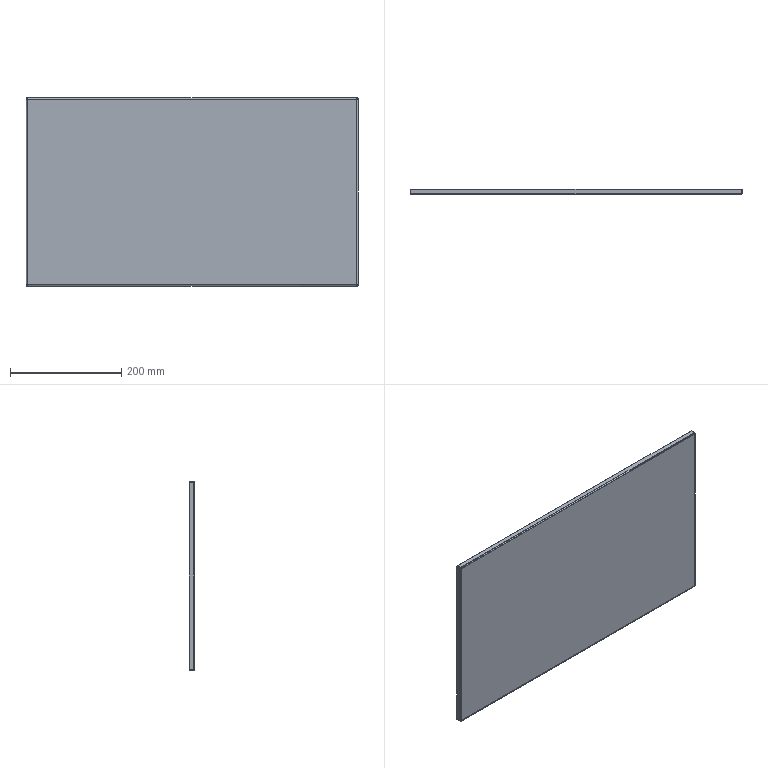Part | SolidWorks | features EdgeFlange 1, FlatPattern 1, SMBaseFlange 1, SheetMetal 1 | 1 solid | 38 faces | box 596 x 10 x 338 mm | volume 259798 mm3 | plane 22 | spline 8 | cylinder 8 | commonest cylinder face diameters 2 x4 4.4 x4